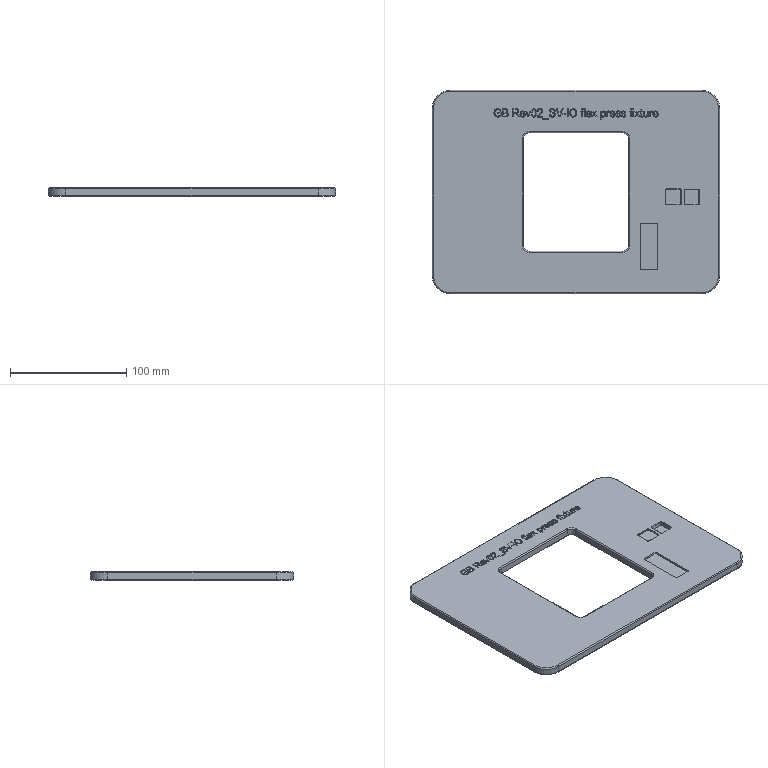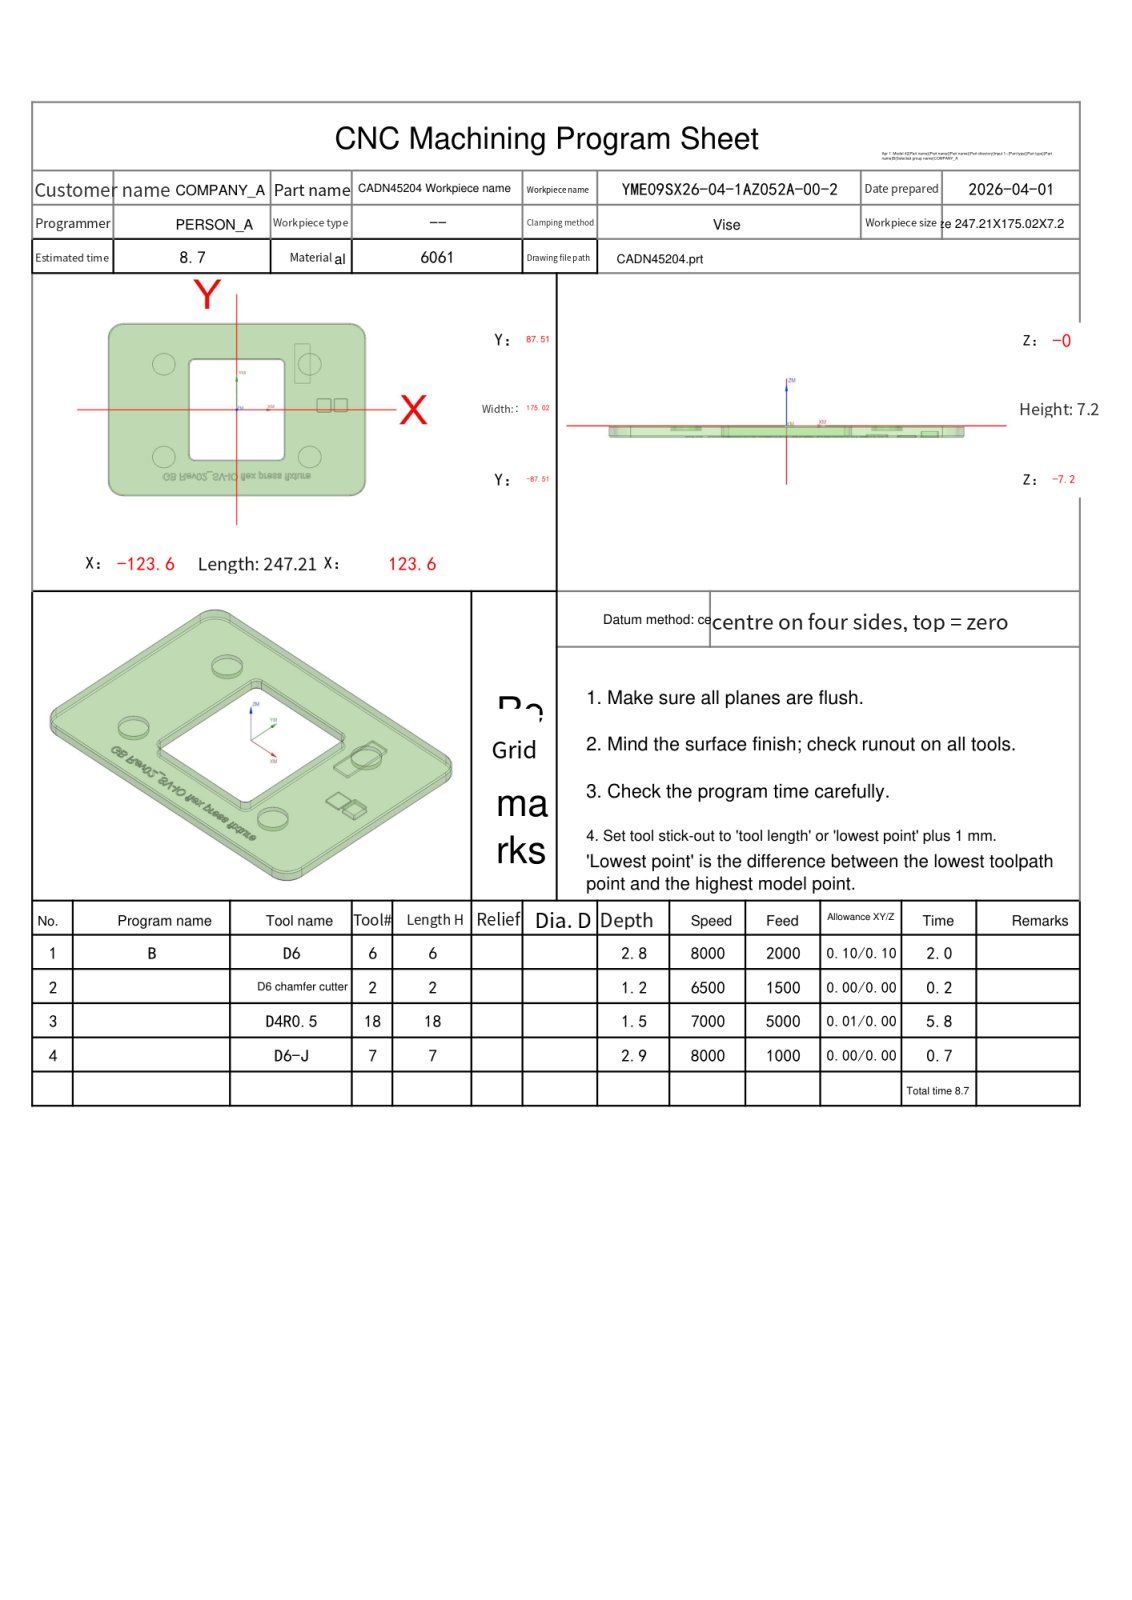NC program | NX | posted by the shop | part box 247.208 x 175.016 x 7.2 mm
Lines 1 to 995 of 22917:
%
O0001
(Machine time: 9.50 MIN)
(===Total Tool:4===)
(T6=D6      D=6.   R=0.   D-  H06 Z=-2.8  )
(T2=D6 chamfer cutter   D=6.   R=0.   D-  H02 Z=-1.2  )
(T18=D4R0.5 D=4.   R=0.5  D-  H18 Z=-1.5  )
(T7=D6-J    D=6.   R=0.   D7  H07 Z=-2.9  )
G80 G90 G17 G49 G40
G91 G28 Z0
M01
N1 T06 M06
(D6  D=6. R=0. H=06 ce=0.10 di=0.10)
G00 G90 G54 X68.687 Y-48.035 M03 S8000
G43 H06 Z10.1
M08
Z1.5
G03 X68.687 Y-48.035 Z.611 I1.313 J2.359 F2000.
X68.687 Y-48.035 Z-.278 I1.313 J2.359
X70. Y-48.375 Z-.35 I1.313 J2.359
X70.4 Y-47.975 I0.0 J.4
X70. Y-47.575 I-.4 J0.0
X69.6 Y-47.975 I0.0 J-.4
X69.839 Y-48.341 I.4 J0.0
G02 X70.124 Y-48.604 I-.242 J-.549
G01 X71.187 Y-50.561
G03 X71.661 Y-50.843 I.475 J.258
X71.975 Y-50.743 I0.0 J.54
X73.4 Y-47.975 I-1.975 J2.768
X70. Y-44.575 I-3.4 J0.0
X66.6 Y-47.975 I0.0 J-3.4
X68.41 Y-50.981 I3.4 J0.0
G02 X68.637 Y-51.192 I-.281 J-.53
G01 X71.266 Y-55.376
G03 X71.774 Y-55.656 I.508 J.319
G01 X71.92 Y-55.639
G03 X77.9 Y-47.975 I-1.92 J7.663
X70. Y-40.075 I-7.9 J0.0
X62.1 Y-47.975 I0.0 J-7.9
X70. Y-55.875 I7.9 J0.0
X72.928 Y-55.313 I0.0 J7.9
X73.387 Y-55.113 I-2.928 J7.337
G01 X72.101 Y-52.402
Z1.15
G00 X68.687 Y-48.035
G03 X68.687 Y-48.035 Z.261 I1.313 J2.359
X68.687 Y-48.035 Z-.628 I1.313 J2.359
X70. Y-48.375 Z-.7 I1.313 J2.359
X70.4 Y-47.975 I0.0 J.4
X70. Y-47.575 I-.4 J0.0
X69.6 Y-47.975 I0.0 J-.4
X69.839 Y-48.341 I.4 J0.0
G02 X70.124 Y-48.604 I-.242 J-.549
G01 X71.187 Y-50.561
G03 X71.661 Y-50.843 I.475 J.258
X71.975 Y-50.743 I0.0 J.54
X73.4 Y-47.975 I-1.975 J2.768
X70. Y-44.575 I-3.4 J0.0
X66.6 Y-47.975 I0.0 J-3.4
X68.41 Y-50.981 I3.4 J0.0
G02 X68.637 Y-51.192 I-.281 J-.53
G01 X71.266 Y-55.376
G03 X71.774 Y-55.656 I.508 J.319
G01 X71.92 Y-55.639
G03 X77.9 Y-47.975 I-1.92 J7.663
X70. Y-40.075 I-7.9 J0.0
X62.1 Y-47.975 I0.0 J-7.9
X70. Y-55.875 I7.9 J0.0
X72.928 Y-55.313 I0.0 J7.9
X73.387 Y-55.113 I-2.928 J7.337
G01 X72.101 Y-52.402
Z.8
G00 X68.687 Y-48.035
G03 X68.687 Y-48.035 Z-.089 I1.313 J2.359
X68.687 Y-48.035 Z-.978 I1.313 J2.359
X70. Y-48.375 Z-1.05 I1.313 J2.359
X70.4 Y-47.975 I0.0 J.4
X70. Y-47.575 I-.4 J0.0
X69.6 Y-47.975 I0.0 J-.4
X69.839 Y-48.341 I.4 J0.0
G02 X70.124 Y-48.604 I-.242 J-.549
G01 X71.187 Y-50.561
G03 X71.661 Y-50.843 I.475 J.258
X71.975 Y-50.743 I0.0 J.54
X73.4 Y-47.975 I-1.975 J2.768
X70. Y-44.575 I-3.4 J0.0
X66.6 Y-47.975 I0.0 J-3.4
X68.41 Y-50.981 I3.4 J0.0
G02 X68.637 Y-51.192 I-.281 J-.53
G01 X71.266 Y-55.376
G03 X71.774 Y-55.656 I.508 J.319
G01 X71.92 Y-55.639
G03 X77.9 Y-47.975 I-1.92 J7.663
X70. Y-40.075 I-7.9 J0.0
X62.1 Y-47.975 I0.0 J-7.9
X70. Y-55.875 I7.9 J0.0
X72.928 Y-55.313 I0.0 J7.9
X73.387 Y-55.113 I-2.928 J7.337
G01 X72.101 Y-52.402
Z.45
G00 X68.687 Y-48.035
G03 X68.687 Y-48.035 Z-.439 I1.313 J2.359
X68.687 Y-48.035 Z-1.328 I1.313 J2.359
X70. Y-48.375 Z-1.4 I1.313 J2.359
X70.4 Y-47.975 I0.0 J.4
X70. Y-47.575 I-.4 J0.0
X69.6 Y-47.975 I0.0 J-.4
X69.839 Y-48.341 I.4 J0.0
G02 X70.124 Y-48.604 I-.242 J-.549
G01 X71.187 Y-50.561
G03 X71.661 Y-50.843 I.475 J.258
X71.975 Y-50.743 I0.0 J.54
X73.4 Y-47.975 I-1.975 J2.768
X70. Y-44.575 I-3.4 J0.0
X66.6 Y-47.975 I0.0 J-3.4
X68.41 Y-50.981 I3.4 J0.0
G02 X68.637 Y-51.192 I-.281 J-.53
G01 X71.266 Y-55.376
G03 X71.774 Y-55.656 I.508 J.319
G01 X71.92 Y-55.639
G03 X77.9 Y-47.975 I-1.92 J7.663
X70. Y-40.075 I-7.9 J0.0
X62.1 Y-47.975 I0.0 J-7.9
X70. Y-55.875 I7.9 J0.0
X72.928 Y-55.313 I0.0 J7.9
X73.387 Y-55.113 I-2.928 J7.337
G01 X72.101 Y-52.402
Z.1
G00 X68.687 Y-48.035
G03 X68.687 Y-48.035 Z-.789 I1.313 J2.359
X68.687 Y-48.035 Z-1.678 I1.313 J2.359
X70. Y-48.375 Z-1.75 I1.313 J2.359
X70.4 Y-47.975 I0.0 J.4
X70. Y-47.575 I-.4 J0.0
X69.6 Y-47.975 I0.0 J-.4
X69.839 Y-48.341 I.4 J0.0
G02 X70.124 Y-48.604 I-.242 J-.549
G01 X71.187 Y-50.561
G03 X71.661 Y-50.843 I.475 J.258
X71.975 Y-50.743 I0.0 J.54
X73.4 Y-47.975 I-1.975 J2.768
X70. Y-44.575 I-3.4 J0.0
X66.6 Y-47.975 I0.0 J-3.4
X68.41 Y-50.981 I3.4 J0.0
G02 X68.637 Y-51.192 I-.281 J-.53
G01 X71.266 Y-55.376
G03 X71.774 Y-55.656 I.508 J.319
G01 X71.92 Y-55.639
G03 X77.9 Y-47.975 I-1.92 J7.663
X70. Y-40.075 I-7.9 J0.0
X62.1 Y-47.975 I0.0 J-7.9
X70. Y-55.875 I7.9 J0.0
X72.928 Y-55.313 I0.0 J7.9
X73.387 Y-55.113 I-2.928 J7.337
G01 X72.101 Y-52.402
Z-.25
G00 X68.687 Y-48.035
G03 X68.687 Y-48.035 Z-1.139 I1.313 J2.359
X68.687 Y-48.035 Z-2.028 I1.313 J2.359
X70. Y-48.375 Z-2.1 I1.313 J2.359
X70.4 Y-47.975 I0.0 J.4
X70. Y-47.575 I-.4 J0.0
X69.6 Y-47.975 I0.0 J-.4
X69.839 Y-48.341 I.4 J0.0
G02 X70.124 Y-48.604 I-.242 J-.549
G01 X71.187 Y-50.561
G03 X71.661 Y-50.843 I.475 J.258
X71.975 Y-50.743 I0.0 J.54
X73.4 Y-47.975 I-1.975 J2.768
X70. Y-44.575 I-3.4 J0.0
X66.6 Y-47.975 I0.0 J-3.4
X68.41 Y-50.981 I3.4 J0.0
G02 X68.637 Y-51.192 I-.281 J-.53
G01 X71.266 Y-55.376
G03 X71.774 Y-55.656 I.508 J.319
G01 X71.92 Y-55.639
G03 X77.9 Y-47.975 I-1.92 J7.663
X70. Y-40.075 I-7.9 J0.0
X62.1 Y-47.975 I0.0 J-7.9
X70. Y-55.875 I7.9 J0.0
X72.928 Y-55.313 I0.0 J7.9
X73.387 Y-55.113 I-2.928 J7.337
G01 X72.101 Y-52.402
Z-.6
G00 X68.687 Y-48.035
G03 X68.687 Y-48.035 Z-1.489 I1.313 J2.359
X68.687 Y-48.035 Z-2.378 I1.313 J2.359
X70. Y-48.375 Z-2.45 I1.313 J2.359
X70.4 Y-47.975 I0.0 J.4
X70. Y-47.575 I-.4 J0.0
X69.6 Y-47.975 I0.0 J-.4
X69.839 Y-48.341 I.4 J0.0
G02 X70.124 Y-48.604 I-.242 J-.549
G01 X71.187 Y-50.561
G03 X71.661 Y-50.843 I.475 J.258
X71.975 Y-50.743 I0.0 J.54
X73.4 Y-47.975 I-1.975 J2.768
X70. Y-44.575 I-3.4 J0.0
X66.6 Y-47.975 I0.0 J-3.4
X68.41 Y-50.981 I3.4 J0.0
G02 X68.637 Y-51.192 I-.281 J-.53
G01 X71.266 Y-55.376
G03 X71.774 Y-55.656 I.508 J.319
G01 X71.92 Y-55.639
G03 X77.9 Y-47.975 I-1.92 J7.663
X70. Y-40.075 I-7.9 J0.0
X62.1 Y-47.975 I0.0 J-7.9
X70. Y-55.875 I7.9 J0.0
X72.928 Y-55.313 I0.0 J7.9
X73.387 Y-55.113 I-2.928 J7.337
G01 X72.101 Y-52.402
Z-.95
G00 X68.687 Y-48.035
G03 X68.687 Y-48.035 Z-1.839 I1.313 J2.359
X68.687 Y-48.035 Z-2.728 I1.313 J2.359
X70. Y-48.375 Z-2.8 I1.313 J2.359
X70.4 Y-47.975 I0.0 J.4
X70. Y-47.575 I-.4 J0.0
X69.6 Y-47.975 I0.0 J-.4
X69.839 Y-48.341 I.4 J0.0
G02 X70.124 Y-48.604 I-.242 J-.549
G01 X71.187 Y-50.561
G03 X71.661 Y-50.843 I.475 J.258
X71.975 Y-50.743 I0.0 J.54
X73.4 Y-47.975 I-1.975 J2.768
X70. Y-44.575 I-3.4 J0.0
X66.6 Y-47.975 I0.0 J-3.4
X68.41 Y-50.981 I3.4 J0.0
G02 X68.637 Y-51.192 I-.281 J-.53
G01 X71.266 Y-55.376
G03 X71.774 Y-55.656 I.508 J.319
G01 X71.92 Y-55.639
G03 X77.9 Y-47.975 I-1.92 J7.663
X70. Y-40.075 I-7.9 J0.0
X62.1 Y-47.975 I0.0 J-7.9
X70. Y-55.875 I7.9 J0.0
X72.928 Y-55.313 I0.0 J7.9
X73.387 Y-55.113 I-2.928 J7.337
G01 X72.101 Y-52.402
Z-1.3
G00 Z10.1
X71.313 Y46.084
Z1.5
G03 X71.313 Y46.084 Z.611 I-1.313 J-2.359
X71.313 Y46.084 Z-.278 I-1.313 J-2.359
X70. Y46.425 Z-.35 I-1.313 J-2.359
X69.6 Y46.025 I0.0 J-.4
X70. Y45.625 I.4 J0.0
X70.4 Y46.025 I0.0 J.4
X70.161 Y46.391 I-.4 J0.0
G02 X69.876 Y46.653 I.242 J.549
G01 X68.813 Y48.61
G03 X68.339 Y48.893 I-.475 J-.258
X68.025 Y48.792 I0.0 J-.54
X66.6 Y46.025 I1.975 J-2.768
X70. Y42.625 I3.4 J0.0
X73.4 Y46.025 I0.0 J3.4
X71.59 Y49.03 I-3.4 J0.0
G02 X71.363 Y49.241 I.281 J.53
G01 X68.734 Y53.425
G03 X68.226 Y53.706 I-.508 J-.319
G01 X68.08 Y53.688
G03 X62.1 Y46.025 I1.92 J-7.663
X70. Y38.125 I7.9 J0.0
X77.9 Y46.025 I0.0 J7.9
X70. Y53.925 I-7.9 J0.0
X67.072 Y53.362 I0.0 J-7.9
X66.613 Y53.162 I2.928 J-7.337
G01 X67.899 Y50.452
Z1.15
G00 X71.313 Y46.084
G03 X71.313 Y46.084 Z.261 I-1.313 J-2.359
X71.313 Y46.084 Z-.628 I-1.313 J-2.359
X70. Y46.425 Z-.7 I-1.313 J-2.359
X69.6 Y46.025 I0.0 J-.4
X70. Y45.625 I.4 J0.0
X70.4 Y46.025 I0.0 J.4
X70.161 Y46.391 I-.4 J0.0
G02 X69.876 Y46.653 I.242 J.549
G01 X68.813 Y48.61
G03 X68.339 Y48.893 I-.475 J-.258
X68.025 Y48.792 I0.0 J-.54
X66.6 Y46.025 I1.975 J-2.768
X70. Y42.625 I3.4 J0.0
X73.4 Y46.025 I0.0 J3.4
X71.59 Y49.03 I-3.4 J0.0
G02 X71.363 Y49.241 I.281 J.53
G01 X68.734 Y53.425
G03 X68.226 Y53.706 I-.508 J-.319
G01 X68.08 Y53.688
G03 X62.1 Y46.025 I1.92 J-7.663
X70. Y38.125 I7.9 J0.0
X77.9 Y46.025 I0.0 J7.9
X70. Y53.925 I-7.9 J0.0
X67.072 Y53.362 I0.0 J-7.9
X66.613 Y53.162 I2.928 J-7.337
G01 X67.899 Y50.452
Z.8
G00 X71.313 Y46.084
G03 X71.313 Y46.084 Z-.089 I-1.313 J-2.359
X71.313 Y46.084 Z-.978 I-1.313 J-2.359
X70. Y46.425 Z-1.05 I-1.313 J-2.359
X69.6 Y46.025 I0.0 J-.4
X70. Y45.625 I.4 J0.0
X70.4 Y46.025 I0.0 J.4
X70.161 Y46.391 I-.4 J0.0
G02 X69.876 Y46.653 I.242 J.549
G01 X68.813 Y48.61
G03 X68.339 Y48.893 I-.475 J-.258
X68.025 Y48.792 I0.0 J-.54
X66.6 Y46.025 I1.975 J-2.768
X70. Y42.625 I3.4 J0.0
X73.4 Y46.025 I0.0 J3.4
X71.59 Y49.03 I-3.4 J0.0
G02 X71.363 Y49.241 I.281 J.53
G01 X68.734 Y53.425
G03 X68.226 Y53.706 I-.508 J-.319
G01 X68.08 Y53.688
G03 X62.1 Y46.025 I1.92 J-7.663
X70. Y38.125 I7.9 J0.0
X77.9 Y46.025 I0.0 J7.9
X70. Y53.925 I-7.9 J0.0
X67.072 Y53.362 I0.0 J-7.9
X66.613 Y53.162 I2.928 J-7.337
G01 X67.899 Y50.452
Z.45
G00 X71.313 Y46.084
G03 X71.313 Y46.084 Z-.439 I-1.313 J-2.359
X71.313 Y46.084 Z-1.328 I-1.313 J-2.359
X70. Y46.425 Z-1.4 I-1.313 J-2.359
X69.6 Y46.025 I0.0 J-.4
X70. Y45.625 I.4 J0.0
X70.4 Y46.025 I0.0 J.4
X70.161 Y46.391 I-.4 J0.0
G02 X69.876 Y46.653 I.242 J.549
G01 X68.813 Y48.61
G03 X68.339 Y48.893 I-.475 J-.258
X68.025 Y48.792 I0.0 J-.54
X66.6 Y46.025 I1.975 J-2.768
X70. Y42.625 I3.4 J0.0
X73.4 Y46.025 I0.0 J3.4
X71.59 Y49.03 I-3.4 J0.0
G02 X71.363 Y49.241 I.281 J.53
G01 X68.734 Y53.425
G03 X68.226 Y53.706 I-.508 J-.319
G01 X68.08 Y53.688
G03 X62.1 Y46.025 I1.92 J-7.663
X70. Y38.125 I7.9 J0.0
X77.9 Y46.025 I0.0 J7.9
X70. Y53.925 I-7.9 J0.0
X67.072 Y53.362 I0.0 J-7.9
X66.613 Y53.162 I2.928 J-7.337
G01 X67.899 Y50.452
Z.1
G00 X71.313 Y46.084
G03 X71.313 Y46.084 Z-.789 I-1.313 J-2.359
X71.313 Y46.084 Z-1.678 I-1.313 J-2.359
X70. Y46.425 Z-1.75 I-1.313 J-2.359
X69.6 Y46.025 I0.0 J-.4
X70. Y45.625 I.4 J0.0
X70.4 Y46.025 I0.0 J.4
X70.161 Y46.391 I-.4 J0.0
G02 X69.876 Y46.653 I.242 J.549
G01 X68.813 Y48.61
G03 X68.339 Y48.893 I-.475 J-.258
X68.025 Y48.792 I0.0 J-.54
X66.6 Y46.025 I1.975 J-2.768
X70. Y42.625 I3.4 J0.0
X73.4 Y46.025 I0.0 J3.4
X71.59 Y49.03 I-3.4 J0.0
G02 X71.363 Y49.241 I.281 J.53
G01 X68.734 Y53.425
G03 X68.226 Y53.706 I-.508 J-.319
G01 X68.08 Y53.688
G03 X62.1 Y46.025 I1.92 J-7.663
X70. Y38.125 I7.9 J0.0
X77.9 Y46.025 I0.0 J7.9
X70. Y53.925 I-7.9 J0.0
X67.072 Y53.362 I0.0 J-7.9
X66.613 Y53.162 I2.928 J-7.337
G01 X67.899 Y50.452
Z-.25
G00 X71.313 Y46.084
G03 X71.313 Y46.084 Z-1.139 I-1.313 J-2.359
X71.313 Y46.084 Z-2.028 I-1.313 J-2.359
X70. Y46.425 Z-2.1 I-1.313 J-2.359
X69.6 Y46.025 I0.0 J-.4
X70. Y45.625 I.4 J0.0
X70.4 Y46.025 I0.0 J.4
X70.161 Y46.391 I-.4 J0.0
G02 X69.876 Y46.653 I.242 J.549
G01 X68.813 Y48.61
G03 X68.339 Y48.893 I-.475 J-.258
X68.025 Y48.792 I0.0 J-.54
X66.6 Y46.025 I1.975 J-2.768
X70. Y42.625 I3.4 J0.0
X73.4 Y46.025 I0.0 J3.4
X71.59 Y49.03 I-3.4 J0.0
G02 X71.363 Y49.241 I.281 J.53
G01 X68.734 Y53.425
G03 X68.226 Y53.706 I-.508 J-.319
G01 X68.08 Y53.688
G03 X62.1 Y46.025 I1.92 J-7.663
X70. Y38.125 I7.9 J0.0
X77.9 Y46.025 I0.0 J7.9
X70. Y53.925 I-7.9 J0.0
X67.072 Y53.362 I0.0 J-7.9
X66.613 Y53.162 I2.928 J-7.337
G01 X67.899 Y50.452
Z-.6
G00 X71.313 Y46.084
G03 X71.313 Y46.084 Z-1.489 I-1.313 J-2.359
X71.313 Y46.084 Z-2.378 I-1.313 J-2.359
X70. Y46.425 Z-2.45 I-1.313 J-2.359
X69.6 Y46.025 I0.0 J-.4
X70. Y45.625 I.4 J0.0
X70.4 Y46.025 I0.0 J.4
X70.161 Y46.391 I-.4 J0.0
G02 X69.876 Y46.653 I.242 J.549
G01 X68.813 Y48.61
G03 X68.339 Y48.893 I-.475 J-.258
X68.025 Y48.792 I0.0 J-.54
X66.6 Y46.025 I1.975 J-2.768
X70. Y42.625 I3.4 J0.0
X73.4 Y46.025 I0.0 J3.4
X71.59 Y49.03 I-3.4 J0.0
G02 X71.363 Y49.241 I.281 J.53
G01 X68.734 Y53.425
G03 X68.226 Y53.706 I-.508 J-.319
G01 X68.08 Y53.688
G03 X62.1 Y46.025 I1.92 J-7.663
X70. Y38.125 I7.9 J0.0
X77.9 Y46.025 I0.0 J7.9
X70. Y53.925 I-7.9 J0.0
X67.072 Y53.362 I0.0 J-7.9
X66.613 Y53.162 I2.928 J-7.337
G01 X67.899 Y50.452
Z-.95
G00 X71.313 Y46.084
G03 X71.313 Y46.084 Z-1.839 I-1.313 J-2.359
X71.313 Y46.084 Z-2.728 I-1.313 J-2.359
X70. Y46.425 Z-2.8 I-1.313 J-2.359
X69.6 Y46.025 I0.0 J-.4
X70. Y45.625 I.4 J0.0
X70.4 Y46.025 I0.0 J.4
X70.161 Y46.391 I-.4 J0.0
G02 X69.876 Y46.653 I.242 J.549
G01 X68.813 Y48.61
G03 X68.339 Y48.893 I-.475 J-.258
X68.025 Y48.792 I0.0 J-.54
X66.6 Y46.025 I1.975 J-2.768
X70. Y42.625 I3.4 J0.0
X73.4 Y46.025 I0.0 J3.4
X71.59 Y49.03 I-3.4 J0.0
G02 X71.363 Y49.241 I.281 J.53
G01 X68.734 Y53.425
G03 X68.226 Y53.706 I-.508 J-.319
G01 X68.08 Y53.688
G03 X62.1 Y46.025 I1.92 J-7.663
X70. Y38.125 I7.9 J0.0
X77.9 Y46.025 I0.0 J7.9
X70. Y53.925 I-7.9 J0.0
X67.072 Y53.362 I0.0 J-7.9
X66.613 Y53.162 I2.928 J-7.337
G01 X67.899 Y50.452
Z-1.3
G00 Z10.1
X-68.687 Y46.084
Z1.5
G03 X-68.687 Y46.084 Z.611 I-1.313 J-2.359
X-68.687 Y46.084 Z-.278 I-1.313 J-2.359
X-70. Y46.425 Z-.35 I-1.313 J-2.359
X-70.4 Y46.025 I0.0 J-.4
X-70. Y45.625 I.4 J0.0
X-69.6 Y46.025 I0.0 J.4
X-69.839 Y46.391 I-.4 J0.0
G02 X-70.124 Y46.653 I.242 J.549
G01 X-71.187 Y48.61
G03 X-71.661 Y48.893 I-.475 J-.258
X-71.975 Y48.792 I0.0 J-.54
X-73.4 Y46.025 I1.975 J-2.768
X-70. Y42.625 I3.4 J0.0
X-66.6 Y46.025 I0.0 J3.4
X-68.41 Y49.03 I-3.4 J0.0
G02 X-68.637 Y49.241 I.281 J.53
G01 X-71.266 Y53.425
G03 X-71.774 Y53.706 I-.508 J-.319
G01 X-71.92 Y53.688
G03 X-77.9 Y46.025 I1.92 J-7.663
X-70. Y38.125 I7.9 J0.0
X-62.1 Y46.025 I0.0 J7.9
X-70. Y53.925 I-7.9 J0.0
X-72.928 Y53.362 I0.0 J-7.9
X-73.387 Y53.162 I2.928 J-7.337
G01 X-72.101 Y50.452
Z1.15
G00 X-68.687 Y46.084
G03 X-68.687 Y46.084 Z.261 I-1.313 J-2.359
X-68.687 Y46.084 Z-.628 I-1.313 J-2.359
X-70. Y46.425 Z-.7 I-1.313 J-2.359
X-70.4 Y46.025 I0.0 J-.4
X-70. Y45.625 I.4 J0.0
X-69.6 Y46.025 I0.0 J.4
X-69.839 Y46.391 I-.4 J0.0
G02 X-70.124 Y46.653 I.242 J.549
G01 X-71.187 Y48.61
G03 X-71.661 Y48.893 I-.475 J-.258
X-71.975 Y48.792 I0.0 J-.54
X-73.4 Y46.025 I1.975 J-2.768
X-70. Y42.625 I3.4 J0.0
X-66.6 Y46.025 I0.0 J3.4
X-68.41 Y49.03 I-3.4 J0.0
G02 X-68.637 Y49.241 I.281 J.53
G01 X-71.266 Y53.425
G03 X-71.774 Y53.706 I-.508 J-.319
G01 X-71.92 Y53.688
G03 X-77.9 Y46.025 I1.92 J-7.663
X-70. Y38.125 I7.9 J0.0
X-62.1 Y46.025 I0.0 J7.9
X-70. Y53.925 I-7.9 J0.0
X-72.928 Y53.362 I0.0 J-7.9
X-73.387 Y53.162 I2.928 J-7.337
G01 X-72.101 Y50.452
Z.8
G00 X-68.687 Y46.084
G03 X-68.687 Y46.084 Z-.089 I-1.313 J-2.359
X-68.687 Y46.084 Z-.978 I-1.313 J-2.359
X-70. Y46.425 Z-1.05 I-1.313 J-2.359
X-70.4 Y46.025 I0.0 J-.4
X-70. Y45.625 I.4 J0.0
X-69.6 Y46.025 I0.0 J.4
X-69.839 Y46.391 I-.4 J0.0
G02 X-70.124 Y46.653 I.242 J.549
G01 X-71.187 Y48.61
G03 X-71.661 Y48.893 I-.475 J-.258
X-71.975 Y48.792 I0.0 J-.54
X-73.4 Y46.025 I1.975 J-2.768
X-70. Y42.625 I3.4 J0.0
X-66.6 Y46.025 I0.0 J3.4
X-68.41 Y49.03 I-3.4 J0.0
G02 X-68.637 Y49.241 I.281 J.53
G01 X-71.266 Y53.425
G03 X-71.774 Y53.706 I-.508 J-.319
G01 X-71.92 Y53.688
G03 X-77.9 Y46.025 I1.92 J-7.663
X-70. Y38.125 I7.9 J0.0
X-62.1 Y46.025 I0.0 J7.9
X-70. Y53.925 I-7.9 J0.0
X-72.928 Y53.362 I0.0 J-7.9
X-73.387 Y53.162 I2.928 J-7.337
G01 X-72.101 Y50.452
Z.45
G00 X-68.687 Y46.084
G03 X-68.687 Y46.084 Z-.439 I-1.313 J-2.359
X-68.687 Y46.084 Z-1.328 I-1.313 J-2.359
X-70. Y46.425 Z-1.4 I-1.313 J-2.359
X-70.4 Y46.025 I0.0 J-.4
X-70. Y45.625 I.4 J0.0
X-69.6 Y46.025 I0.0 J.4
X-69.839 Y46.391 I-.4 J0.0
G02 X-70.124 Y46.653 I.242 J.549
G01 X-71.187 Y48.61
G03 X-71.661 Y48.893 I-.475 J-.258
X-71.975 Y48.792 I0.0 J-.54
X-73.4 Y46.025 I1.975 J-2.768
X-70. Y42.625 I3.4 J0.0
X-66.6 Y46.025 I0.0 J3.4
X-68.41 Y49.03 I-3.4 J0.0
G02 X-68.637 Y49.241 I.281 J.53
G01 X-71.266 Y53.425
G03 X-71.774 Y53.706 I-.508 J-.319
G01 X-71.92 Y53.688
G03 X-77.9 Y46.025 I1.92 J-7.663
X-70. Y38.125 I7.9 J0.0
X-62.1 Y46.025 I0.0 J7.9
X-70. Y53.925 I-7.9 J0.0
X-72.928 Y53.362 I0.0 J-7.9
X-73.387 Y53.162 I2.928 J-7.337
G01 X-72.101 Y50.452
Z.1
G00 X-68.687 Y46.084
G03 X-68.687 Y46.084 Z-.789 I-1.313 J-2.359
X-68.687 Y46.084 Z-1.678 I-1.313 J-2.359
X-70. Y46.425 Z-1.75 I-1.313 J-2.359
X-70.4 Y46.025 I0.0 J-.4
X-70. Y45.625 I.4 J0.0
X-69.6 Y46.025 I0.0 J.4
X-69.839 Y46.391 I-.4 J0.0
G02 X-70.124 Y46.653 I.242 J.549
G01 X-71.187 Y48.61
G03 X-71.661 Y48.893 I-.475 J-.258
X-71.975 Y48.792 I0.0 J-.54
X-73.4 Y46.025 I1.975 J-2.768
X-70. Y42.625 I3.4 J0.0
X-66.6 Y46.025 I0.0 J3.4
X-68.41 Y49.03 I-3.4 J0.0
G02 X-68.637 Y49.241 I.281 J.53
G01 X-71.266 Y53.425
G03 X-71.774 Y53.706 I-.508 J-.319
G01 X-71.92 Y53.688
G03 X-77.9 Y46.025 I1.92 J-7.663
X-70. Y38.125 I7.9 J0.0
X-62.1 Y46.025 I0.0 J7.9
X-70. Y53.925 I-7.9 J0.0
X-72.928 Y53.362 I0.0 J-7.9
X-73.387 Y53.162 I2.928 J-7.337
G01 X-72.101 Y50.452
Z-.25
G00 X-68.687 Y46.084
G03 X-68.687 Y46.084 Z-1.139 I-1.313 J-2.359
X-68.687 Y46.084 Z-2.028 I-1.313 J-2.359
X-70. Y46.425 Z-2.1 I-1.313 J-2.359
X-70.4 Y46.025 I0.0 J-.4
X-70. Y45.625 I.4 J0.0
X-69.6 Y46.025 I0.0 J.4
X-69.839 Y46.391 I-.4 J0.0
G02 X-70.124 Y46.653 I.242 J.549
G01 X-71.187 Y48.61
G03 X-71.661 Y48.893 I-.475 J-.258
X-71.975 Y48.792 I0.0 J-.54
X-73.4 Y46.025 I1.975 J-2.768
X-70. Y42.625 I3.4 J0.0
X-66.6 Y46.025 I0.0 J3.4
X-68.41 Y49.03 I-3.4 J0.0
G02 X-68.637 Y49.241 I.281 J.53
G01 X-71.266 Y53.425
G03 X-71.774 Y53.706 I-.508 J-.319
G01 X-71.92 Y53.688
G03 X-77.9 Y46.025 I1.92 J-7.663
X-70. Y38.125 I7.9 J0.0
X-62.1 Y46.025 I0.0 J7.9
X-70. Y53.925 I-7.9 J0.0
X-72.928 Y53.362 I0.0 J-7.9
X-73.387 Y53.162 I2.928 J-7.337
G01 X-72.101 Y50.452
Z-.6
G00 X-68.687 Y46.084
G03 X-68.687 Y46.084 Z-1.489 I-1.313 J-2.359
X-68.687 Y46.084 Z-2.378 I-1.313 J-2.359
X-70. Y46.425 Z-2.45 I-1.313 J-2.359
X-70.4 Y46.025 I0.0 J-.4
X-70. Y45.625 I.4 J0.0
X-69.6 Y46.025 I0.0 J.4
X-69.839 Y46.391 I-.4 J0.0
G02 X-70.124 Y46.653 I.242 J.549
G01 X-71.187 Y48.61
G03 X-71.661 Y48.893 I-.475 J-.258
X-71.975 Y48.792 I0.0 J-.54
X-73.4 Y46.025 I1.975 J-2.768
X-70. Y42.625 I3.4 J0.0
X-66.6 Y46.025 I0.0 J3.4
X-68.41 Y49.03 I-3.4 J0.0
G02 X-68.637 Y49.241 I.281 J.53
G01 X-71.266 Y53.425
G03 X-71.774 Y53.706 I-.508 J-.319
G01 X-71.92 Y53.688
G03 X-77.9 Y46.025 I1.92 J-7.663
X-70. Y38.125 I7.9 J0.0
X-62.1 Y46.025 I0.0 J7.9
X-70. Y53.925 I-7.9 J0.0
X-72.928 Y53.362 I0.0 J-7.9
X-73.387 Y53.162 I2.928 J-7.337
G01 X-72.101 Y50.452
Z-.95
G00 X-68.687 Y46.084
G03 X-68.687 Y46.084 Z-1.839 I-1.313 J-2.359
X-68.687 Y46.084 Z-2.728 I-1.313 J-2.359
X-70. Y46.425 Z-2.8 I-1.313 J-2.359
X-70.4 Y46.025 I0.0 J-.4
X-70. Y45.625 I.4 J0.0
X-69.6 Y46.025 I0.0 J.4
X-69.839 Y46.391 I-.4 J0.0
G02 X-70.124 Y46.653 I.242 J.549
G01 X-71.187 Y48.61
G03 X-71.661 Y48.893 I-.475 J-.258
X-71.975 Y48.792 I0.0 J-.54
X-73.4 Y46.025 I1.975 J-2.768
X-70. Y42.625 I3.4 J0.0
X-66.6 Y46.025 I0.0 J3.4
X-68.41 Y49.03 I-3.4 J0.0
G02 X-68.637 Y49.241 I.281 J.53
G01 X-71.266 Y53.425
G03 X-71.774 Y53.706 I-.508 J-.319
G01 X-71.92 Y53.688
G03 X-77.9 Y46.025 I1.92 J-7.663
X-70. Y38.125 I7.9 J0.0
X-62.1 Y46.025 I0.0 J7.9
X-70. Y53.925 I-7.9 J0.0
X-72.928 Y53.362 I0.0 J-7.9
X-73.387 Y53.162 I2.928 J-7.337
G01 X-72.101 Y50.452
Z-1.3
G00 Z10.1
X-71.313 Y-48.035
Z1.5
G03 X-71.313 Y-48.035 Z.611 I1.313 J2.359
X-71.313 Y-48.035 Z-.278 I1.313 J2.359
X-70. Y-48.375 Z-.35 I1.313 J2.359
X-69.6 Y-47.975 I0.0 J.4
X-70. Y-47.575 I-.4 J0.0
X-70.4 Y-47.975 I0.0 J-.4
X-70.161 Y-48.341 I.4 J0.0
G02 X-69.876 Y-48.604 I-.242 J-.549
G01 X-68.813 Y-50.561
G03 X-68.339 Y-50.843 I.475 J.258
X-68.025 Y-50.743 I0.0 J.54
X-66.6 Y-47.975 I-1.975 J2.768
X-70. Y-44.575 I-3.4 J0.0
X-73.4 Y-47.975 I0.0 J-3.4
X-71.59 Y-50.981 I3.4 J0.0
G02 X-71.363 Y-51.192 I-.281 J-.53
G01 X-68.734 Y-55.376
G03 X-68.226 Y-55.656 I.508 J.319
G01 X-68.08 Y-55.639
G03 X-62.1 Y-47.975 I-1.92 J7.663
X-70. Y-40.075 I-7.9 J0.0
X-77.9 Y-47.975 I0.0 J-7.9
X-70. Y-55.875 I7.9 J0.0
X-67.072 Y-55.313 I0.0 J7.9
X-66.613 Y-55.113 I-2.928 J7.337
G01 X-67.899 Y-52.402
Z1.15
G00 X-71.313 Y-48.035
G03 X-71.313 Y-48.035 Z.261 I1.313 J2.359
X-71.313 Y-48.035 Z-.628 I1.313 J2.359
X-70. Y-48.375 Z-.7 I1.313 J2.359
X-69.6 Y-47.975 I0.0 J.4
X-70. Y-47.575 I-.4 J0.0
X-70.4 Y-47.975 I0.0 J-.4
X-70.161 Y-48.341 I.4 J0.0
G02 X-69.876 Y-48.604 I-.242 J-.549
G01 X-68.813 Y-50.561
G03 X-68.339 Y-50.843 I.475 J.258
X-68.025 Y-50.743 I0.0 J.54
X-66.6 Y-47.975 I-1.975 J2.768
X-70. Y-44.575 I-3.4 J0.0
X-73.4 Y-47.975 I0.0 J-3.4
X-71.59 Y-50.981 I3.4 J0.0
G02 X-71.363 Y-51.192 I-.281 J-.53
G01 X-68.734 Y-55.376
G03 X-68.226 Y-55.656 I.508 J.319
G01 X-68.08 Y-55.639
G03 X-62.1 Y-47.975 I-1.92 J7.663
X-70. Y-40.075 I-7.9 J0.0
X-77.9 Y-47.975 I0.0 J-7.9
X-70. Y-55.875 I7.9 J0.0
X-67.072 Y-55.313 I0.0 J7.9
X-66.613 Y-55.113 I-2.928 J7.337
G01 X-67.899 Y-52.402
Z.8
G00 X-71.313 Y-48.035
G03 X-71.313 Y-48.035 Z-.089 I1.313 J2.359
X-71.313 Y-48.035 Z-.978 I1.313 J2.359
X-70. Y-48.375 Z-1.05 I1.313 J2.359
X-69.6 Y-47.975 I0.0 J.4
X-70. Y-47.575 I-.4 J0.0
X-70.4 Y-47.975 I0.0 J-.4
X-70.161 Y-48.341 I.4 J0.0
G02 X-69.876 Y-48.604 I-.242 J-.549
G01 X-68.813 Y-50.561
G03 X-68.339 Y-50.843 I.475 J.258
X-68.025 Y-50.743 I0.0 J.54
X-66.6 Y-47.975 I-1.975 J2.768
X-70. Y-44.575 I-3.4 J0.0
X-73.4 Y-47.975 I0.0 J-3.4
X-71.59 Y-50.981 I3.4 J0.0
G02 X-71.363 Y-51.192 I-.281 J-.53
G01 X-68.734 Y-55.376
G03 X-68.226 Y-55.656 I.508 J.319
G01 X-68.08 Y-55.639
G03 X-62.1 Y-47.975 I-1.92 J7.663
X-70. Y-40.075 I-7.9 J0.0
X-77.9 Y-47.975 I0.0 J-7.9
X-70. Y-55.875 I7.9 J0.0
X-67.072 Y-55.313 I0.0 J7.9
X-66.613 Y-55.113 I-2.928 J7.337
G01 X-67.899 Y-52.402
Z.45
G00 X-71.313 Y-48.035
G03 X-71.313 Y-48.035 Z-.439 I1.313 J2.359
X-71.313 Y-48.035 Z-1.328 I1.313 J2.359
X-70. Y-48.375 Z-1.4 I1.313 J2.359
X-69.6 Y-47.975 I0.0 J.4
X-70. Y-47.575 I-.4 J0.0
X-70.4 Y-47.975 I0.0 J-.4
X-70.161 Y-48.341 I.4 J0.0
G02 X-69.876 Y-48.604 I-.242 J-.549
G01 X-68.813 Y-50.561
G03 X-68.339 Y-50.843 I.475 J.258
X-68.025 Y-50.743 I0.0 J.54
X-66.6 Y-47.975 I-1.975 J2.768
X-70. Y-44.575 I-3.4 J0.0
X-73.4 Y-47.975 I0.0 J-3.4
X-71.59 Y-50.981 I3.4 J0.0
G02 X-71.363 Y-51.192 I-.281 J-.53
G01 X-68.734 Y-55.376
G03 X-68.226 Y-55.656 I.508 J.319
G01 X-68.08 Y-55.639
G03 X-62.1 Y-47.975 I-1.92 J7.663
X-70. Y-40.075 I-7.9 J0.0
X-77.9 Y-47.975 I0.0 J-7.9
X-70. Y-55.875 I7.9 J0.0
X-67.072 Y-55.313 I0.0 J7.9
X-66.613 Y-55.113 I-2.928 J7.337
G01 X-67.899 Y-52.402
Z.1
G00 X-71.313 Y-48.035
G03 X-71.313 Y-48.035 Z-.789 I1.313 J2.359
X-71.313 Y-48.035 Z-1.678 I1.313 J2.359
X-70. Y-48.375 Z-1.75 I1.313 J2.359
X-69.6 Y-47.975 I0.0 J.4
X-70. Y-47.575 I-.4 J0.0
X-70.4 Y-47.975 I0.0 J-.4
X-70.161 Y-48.341 I.4 J0.0
G02 X-69.876 Y-48.604 I-.242 J-.549
G01 X-68.813 Y-50.561
G03 X-68.339 Y-50.843 I.475 J.258
X-68.025 Y-50.743 I0.0 J.54
X-66.6 Y-47.975 I-1.975 J2.768
X-70. Y-44.575 I-3.4 J0.0
X-73.4 Y-47.975 I0.0 J-3.4
X-71.59 Y-50.981 I3.4 J0.0
G02 X-71.363 Y-51.192 I-.281 J-.53
G01 X-68.734 Y-55.376
G03 X-68.226 Y-55.656 I.508 J.319
G01 X-68.08 Y-55.639
G03 X-62.1 Y-47.975 I-1.92 J7.663
X-70. Y-40.075 I-7.9 J0.0
X-77.9 Y-47.975 I0.0 J-7.9
X-70. Y-55.875 I7.9 J0.0
X-67.072 Y-55.313 I0.0 J7.9
X-66.613 Y-55.113 I-2.928 J7.337
G01 X-67.899 Y-52.402
Z-.25
G00 X-71.313 Y-48.035
G03 X-71.313 Y-48.035 Z-1.139 I1.313 J2.359
X-71.313 Y-48.035 Z-2.028 I1.313 J2.359
X-70. Y-48.375 Z-2.1 I1.313 J2.359
X-69.6 Y-47.975 I0.0 J.4
X-70. Y-47.575 I-.4 J0.0
X-70.4 Y-47.975 I0.0 J-.4
X-70.161 Y-48.341 I.4 J0.0
G02 X-69.876 Y-48.604 I-.242 J-.549
G01 X-68.813 Y-50.561
G03 X-68.339 Y-50.843 I.475 J.258
X-68.025 Y-50.743 I0.0 J.54
X-66.6 Y-47.975 I-1.975 J2.768
X-70. Y-44.575 I-3.4 J0.0
X-73.4 Y-47.975 I0.0 J-3.4
X-71.59 Y-50.981 I3.4 J0.0
G02 X-71.363 Y-51.192 I-.281 J-.53
G01 X-68.734 Y-55.376
G03 X-68.226 Y-55.656 I.508 J.319
G01 X-68.08 Y-55.639
G03 X-62.1 Y-47.975 I-1.92 J7.663
X-70. Y-40.075 I-7.9 J0.0
X-77.9 Y-47.975 I0.0 J-7.9
X-70. Y-55.875 I7.9 J0.0
X-67.072 Y-55.313 I0.0 J7.9
X-66.613 Y-55.113 I-2.928 J7.337
G01 X-67.899 Y-52.402
Z-.6
G00 X-71.313 Y-48.035
G03 X-71.313 Y-48.035 Z-1.489 I1.313 J2.359
X-71.313 Y-48.035 Z-2.378 I1.313 J2.359
X-70. Y-48.375 Z-2.45 I1.313 J2.359
X-69.6 Y-47.975 I0.0 J.4
X-70. Y-47.575 I-.4 J0.0
X-70.4 Y-47.975 I0.0 J-.4
X-70.161 Y-48.341 I.4 J0.0
G02 X-69.876 Y-48.604 I-.242 J-.549
G01 X-68.813 Y-50.561
G03 X-68.339 Y-50.843 I.475 J.258
X-68.025 Y-50.743 I0.0 J.54
X-66.6 Y-47.975 I-1.975 J2.768
X-70. Y-44.575 I-3.4 J0.0
X-73.4 Y-47.975 I0.0 J-3.4
X-71.59 Y-50.981 I3.4 J0.0
G02 X-71.363 Y-51.192 I-.281 J-.53
G01 X-68.734 Y-55.376
G03 X-68.226 Y-55.656 I.508 J.319
G01 X-68.08 Y-55.639
G03 X-62.1 Y-47.975 I-1.92 J7.663
X-70. Y-40.075 I-7.9 J0.0
X-77.9 Y-47.975 I0.0 J-7.9
X-70. Y-55.875 I7.9 J0.0
X-67.072 Y-55.313 I0.0 J7.9
X-66.613 Y-55.113 I-2.928 J7.337
G01 X-67.899 Y-52.402
Z-.95
G00 X-71.313 Y-48.035
G03 X-71.313 Y-48.035 Z-1.839 I1.313 J2.359
X-71.313 Y-48.035 Z-2.728 I1.313 J2.359
X-70. Y-48.375 Z-2.8 I1.313 J2.359
X-69.6 Y-47.975 I0.0 J.4
X-70. Y-47.575 I-.4 J0.0
X-70.4 Y-47.975 I0.0 J-.4
X-70.161 Y-48.341 I.4 J0.0
G02 X-69.876 Y-48.604 I-.242 J-.549
G01 X-68.813 Y-50.561
G03 X-68.339 Y-50.843 I.475 J.258
X-68.025 Y-50.743 I0.0 J.54
X-66.6 Y-47.975 I-1.975 J2.768
X-70. Y-44.575 I-3.4 J0.0
X-73.4 Y-47.975 I0.0 J-3.4
X-71.59 Y-50.981 I3.4 J0.0
G02 X-71.363 Y-51.192 I-.281 J-.53
G01 X-68.734 Y-55.376
G03 X-68.226 Y-55.656 I.508 J.319
G01 X-68.08 Y-55.639
G03 X-62.1 Y-47.975 I-1.92 J7.663
X-70. Y-40.075 I-7.9 J0.0
X-77.9 Y-47.975 I0.0 J-7.9
X-70. Y-55.875 I7.9 J0.0
X-67.072 Y-55.313 I0.0 J7.9
X-66.613 Y-55.113 I-2.928 J7.337
G01 X-67.899 Y-52.402
Z-1.3
G00 Z10.1
G91 G28 Z0.0
M05
M09
G91 G28 Z0.0
M01
N2 T02 M06
(D6 chamfer cutter  D=6. R=0. H=02 ce=0.00 di=0.00)
G00 G90 G54 X-60.21 Y45.63 M03 S6500
G43 H02 Z50.
M08
Z.207
G01 Z-1.2 F1500.
G03 X-60.022 Y45.924 I-1.587 J1.218
G01 X-59.995 Y45.971
X-60. Y46.025
G03 X-70. Y56.025 I-10. J0.0
X-80. Y46.025 I0.0 J-10.
X-70. Y36.025 I10. J0.0
X-60. Y46.025 I0.0 J10.
G01 X-59.995 Y46.079
X-60.022 Y46.126
G03 X-60.21 Y46.42 I-1.774 J-.923
G01 Z.207
G00 Z10.
Y-48.37
Z.207
G01 Z-1.2
G03 X-60.022 Y-48.076 I-1.587 J1.218
G01 X-59.995 Y-48.03
X-60. Y-47.975
G03 X-70. Y-37.975 I-10. J0.0
X-80. Y-47.975 I0.0 J-10.
X-70. Y-57.975 I10. J0.0
X-60. Y-47.975 I0.0 J10.
G01 X-59.995 Y-47.921
X-60.022 Y-47.874
G03 X-60.21 Y-47.58 I-1.774 J-.923
G01 Z.207
G00 Z10.
X79.79 Y-48.37
Z.207
G01 Z-1.2
G03 X79.978 Y-48.076 I-1.587 J1.218
G01 X80.005 Y-48.03
X80. Y-47.975
G03 X70. Y-37.975 I-10. J0.0
X60. Y-47.975 I0.0 J-10.
X70. Y-57.975 I10. J0.0
X80. Y-47.975 I0.0 J10.
G01 X80.005 Y-47.921
X79.978 Y-47.874
G03 X79.79 Y-47.58 I-1.774 J-.923
G01 Z.207
G00 Z10.
Y45.63
Z.207
G01 Z-1.2
G03 X79.978 Y45.924 I-1.587 J1.218
G01 X80.005 Y45.971
X80. Y46.025
G03 X70. Y56.025 I-10. J0.0
X60. Y46.025 I0.0 J-10.
X70. Y36.025 I10. J0.0
X80. Y46.025 I0.0 J10.
G01 X80.005 Y46.079
X79.978 Y46.126
G03 X79.79 Y46.42 I-1.774 J-.923
G01 Z.207
G00 Z50.
G91 G28 Z0.0
M05
M09
G91 G28 Z0.0
M01